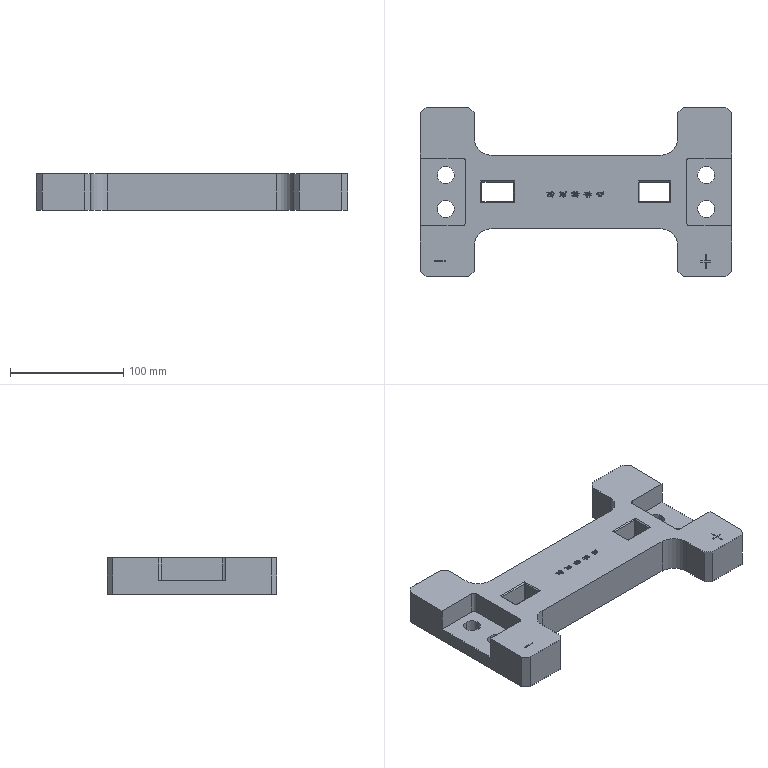Part | 1 solid | 531 faces | box 275 x 150 x 32 mm | volume 699095 mm3 | plane 338 | spline 165 | cylinder 28 | commonest cylinder face diameters 1 x12 15 x8 6 x4 30 x4